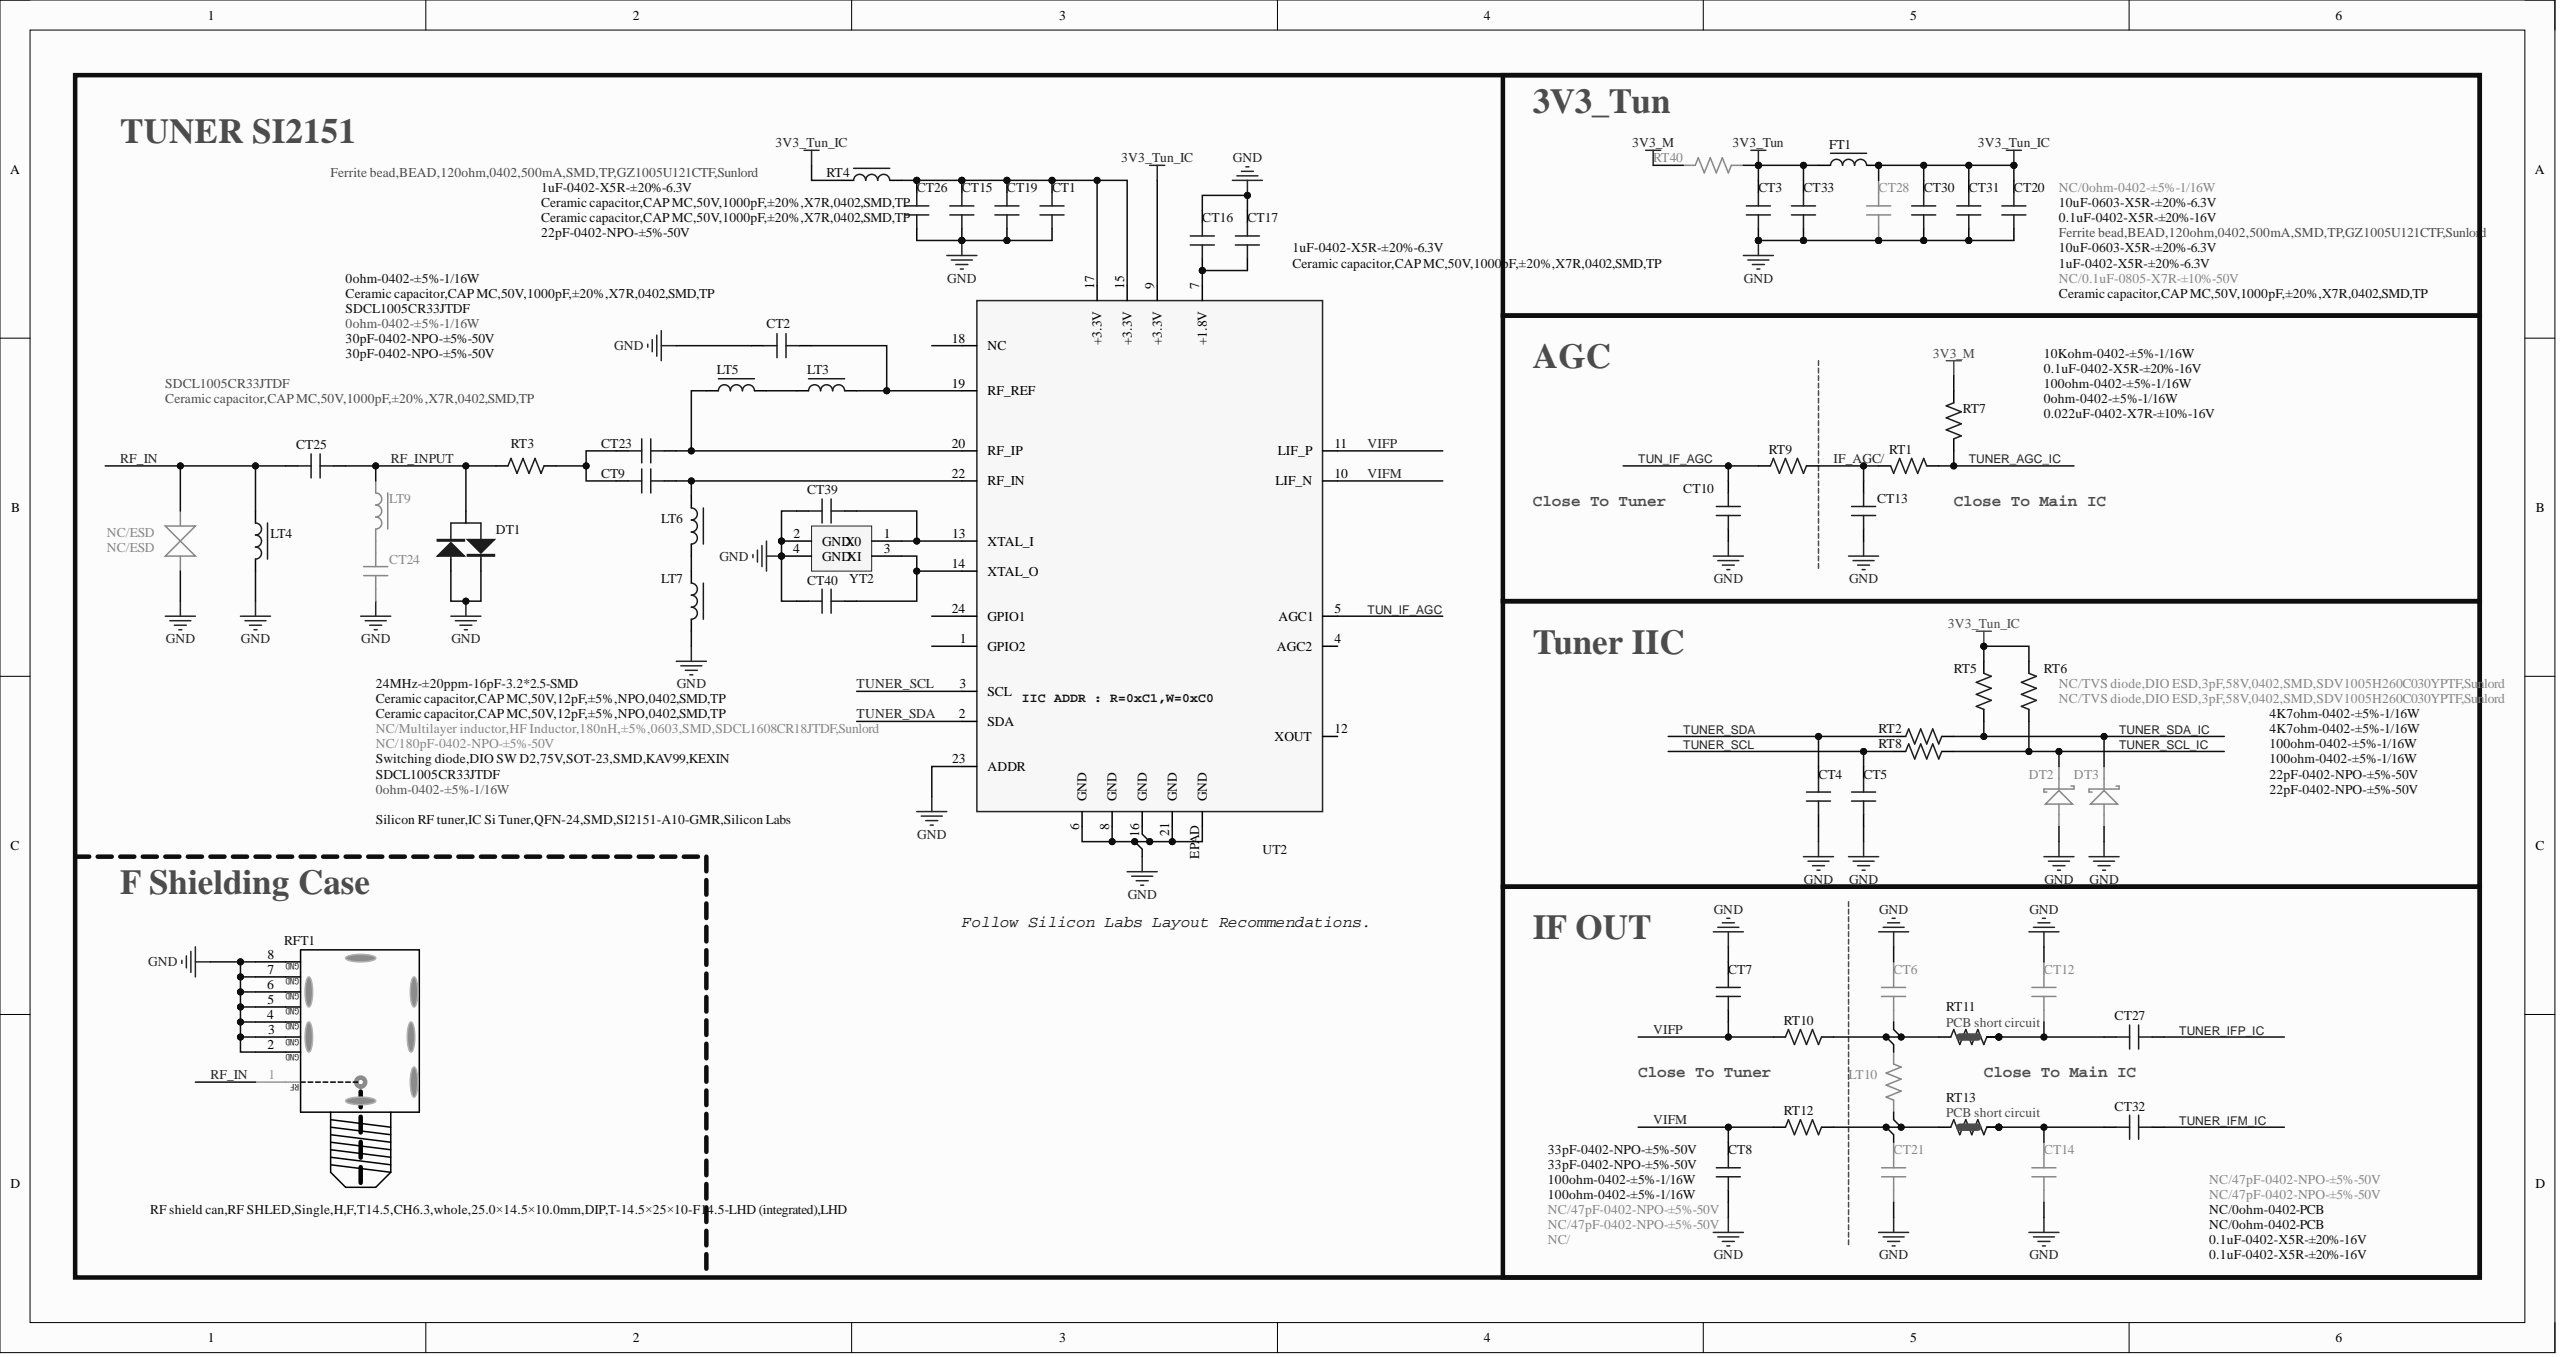Circuit board | Altium Designer | 1029 parts | 642 nets | one sheet of the schematic
Parts on this sheet (reference | value | footprint):
CT1 | Ceramic capacitor,CAP MC,50V,1000pF,±20%,X7R,0402,SMD,TP | C0402
CT2 | Ceramic capacitor,CAP MC,50V,1000pF,±20%,X7R,0402,SMD,TP | C0402
CT3 | 10uF-0603-X5R-±20%-6.3V | C0603
CT4 | 22pF-0402-NPO-±5%-50V | C0402
CT5 | 22pF-0402-NPO-±5%-50V | C0402
CT6 | NC/47pF-0402-NPO-±5%-50V | C0402
CT7 | 33pF-0402-NPO-±5%-50V | C0402
CT8 | 33pF-0402-NPO-±5%-50V | C0402
CT9 | 30pF-0402-NPO-±5%-50V | C0402
CT10 | 0.1uF-0402-X5R-±20%-16V | C0402
CT12 | NC/47pF-0402-NPO-±5%-50V | C0402
CT13 | 0.022uF-0402-X7R-±10%-16V | C0402
CT14 | NC/47pF-0402-NPO-±5%-50V | C0402
CT15 | 1uF-0402-X5R-±20%-6.3V | C0402
CT16 | 1uF-0402-X5R-±20%-6.3V | C0402
CT17 | Ceramic capacitor,CAP MC,50V,1000pF,±20%,X7R,0402,SMD,TP | C0402
CT19 | Ceramic capacitor,CAP MC,50V,1000pF,±20%,X7R,0402,SMD,TP | C0402
CT20 | Ceramic capacitor,CAP MC,50V,1000pF,±20%,X7R,0402,SMD,TP | C0402
CT21 | NC/47pF-0402-NPO-±5%-50V | C0402
CT23 | 30pF-0402-NPO-±5%-50V | C0402
CT24 | NC/180pF-0402-NPO-±5%-50V | C0402
CT25 | Ceramic capacitor,CAP MC,50V,1000pF,±20%,X7R,0402,SMD,TP | C0402
CT26 | 22pF-0402-NPO-±5%-50V | C0402
CT27 | 0.1uF-0402-X5R-±20%-16V | C0402
CT28 | NC/0.1uF-0805-X7R-±10%-50V | C0805
CT30 | 10uF-0603-X5R-±20%-6.3V | C0603
CT31 | 1uF-0402-X5R-±20%-6.3V | C0402
CT32 | 0.1uF-0402-X5R-±20%-16V | C0402
CT33 | 0.1uF-0402-X5R-±20%-16V | C0402
CT39 | Ceramic capacitor,CAP MC,50V,12pF,±5%,NPO,0402,SMD,TP | C0402
CT40 | Ceramic capacitor,CAP MC,50V,12pF,±5%,NPO,0402,SMD,TP | C0402
DT1 | Switching diode,DIO SW D2,75V,SOT-23,SMD,KAV99,KEXIN | SO-23
DT2 | NC/TVS diode,DIO ESD,3pF,58V,0402,SMD,SDV1005H260C030YPTF,Sunlord | DIODE-S0402
DT3 | NC/TVS diode,DIO ESD,3pF,58V,0402,SMD,SDV1005H260C030YPTF,Sunlord | DIODE-S0402
FT1 | Ferrite bead,BEAD,120ohm,0402,500mA,SMD,TP,GZ1005U121CTF,Sunlord | L0402
LT3 | 0ohm-0402-±5%-1/16W | L0402
LT4 | SDCL1005CR33JTDF | L0402
LT5 | SDCL1005CR33JTDF | L0402
LT6 | SDCL1005CR33JTDF | L0402
LT7 | 0ohm-0402-±5%-1/16W | L0402
LT9 | NC/Multilayer inductor,HF Inductor,180nH,±5%,0603,SMD,SDCL1608CR18JTDF,Sunlord | L0603
LT10 | NC/ | R0402
NC/ESD | NC/ESD | ESD
RFT1 | RF shield can,RF SHLED,Single,H,F,T14.5,CH6.3,whole,25.0×14.5×10.0mm,DIP,T-14.5×25×10-F14.5-LHD (integrated),LHD | T-14.5×25×10-F14.5-2
RT1 | 0ohm-0402-±5%-1/16W | R0402
RT2 | 100ohm-0402-±5%-1/16W | R0402
RT3 | 0ohm-0402-±5%-1/16W | R0402
RT4 | Ferrite bead,BEAD,120ohm,0402,500mA,SMD,TP,GZ1005U121CTF,Sunlord | L0402
RT5 | 4K7ohm-0402-±5%-1/16W | R0402
RT6 | 4K7ohm-0402-±5%-1/16W | R0402
RT7 | 10Kohm-0402-±5%-1/16W | R0402
RT8 | 100ohm-0402-±5%-1/16W | R0402
RT9 | 100ohm-0402-±5%-1/16W | R0402
RT10 | 100ohm-0402-±5%-1/16W | R0402
RT11 | NC/0ohm-0402-PCB | R0402SC
RT12 | 100ohm-0402-±5%-1/16W | R0402
RT13 | NC/0ohm-0402-PCB | R0402SC
RT40 | NC/0ohm-0402-±5%-1/16W | R0402
UT2 | Silicon RF tuner,IC Si Tuner,QFN-24,SMD,SI2151-A10-GMR,Silicon Labs | QFN24/0.4-1
YT2 | 24MHz-±20ppm-16pF-3.2*2.5-SMD | XTAL-S-3
Nets of these parts (net: part-pin ...):
VIFP: CT7-2 RT10-1 UT2-11
VIFM: CT8-2 RT12-1 UT2-10
TUNER_SDA_IC: DT3-K RT2-2 RT5-1
TUNER_SDA: CT4-1 RT2-1 UT2-2
TUNER_SCL_IC: DT2-K RT6-1 RT8-2
TUNER_SCL: CT5-1 RT8-1 UT2-3
TUNER_IFP_IC: CT27-1
TUNER_IFM_IC: CT32-2
TUNER_AGC_IC: RT1-2 RT7-1
TUN_IF_AGC: CT10-2 RT9-1 UT2-5
RF_INPUT: CT25-2 DT1-2 LT9-1 RT3-1
RF_IN: CT25-1 LT4-1 NC/ESD-2 RFT1-1
NetLT6_2: LT6-2 LT7-1
NetLT3_1: LT3-1 LT5-2
NetCT40_2: CT40-2 UT2-14 YT2-3
NetCT39_2: CT39-2 UT2-13 YT2-1
NetCT24_1: CT24-1 LT9-2
NetCT23_1: CT23-1 LT5-1 UT2-20
NetCT21_1: CT21-1 LT10-2 RT12-2 RT13-1
NetCT16_2: CT16-2 CT17-2 UT2-7
NetCT14_1: CT14-1 CT32-1 RT13-2 RT13-3
NetCT12_2: CT12-2 CT27-2 RT11-2 RT11-3
NetCT9_2: CT9-2 CT23-2 RT3-2
NetCT9_1: CT9-1 LT6-1 UT2-22
NetCT6_2: CT6-2 LT10-1 RT10-2 RT11-1
NetCT2_2: CT2-2 LT3-2 UT2-19
NetCT1_2: CT1-2 CT15-1 CT19-2 CT26-2 RT4-2 UT2-15 UT2-17
IF_AGC/: CT13-2 RT1-1 RT9-2
GND: CT1-1 CT2-1 CT3-1 CT4-2 CT5-2 CT6-1 CT7-1 CT8-1 CT10-1 CT12-1 CT13-1 CT14-2 CT15-2 CT16-1 CT17-1 CT19-1 CT20-1 CT21-2 CT24-2 CT26-1 CT28-1 CT30-1 CT31-1 CT33-1 CT39-1 CT40-1 DT1-1 DT1-3 DT2-A DT3-A LT4-2 LT7-2 NC/ESD-1 RFT1-2 RFT1-3 RFT1-4 RFT1-5 RFT1-6 RFT1-7 RFT1-8 UT2-6 UT2-8 UT2-16 UT2-21 UT2-23 UT2-EPAD YT2-2 YT2-4
3V3_Tun_IC: CT20-2 CT28-2 CT30-2 CT31-2 FT1-2 RT4-1 RT5-2 RT6-2 UT2-9
3V3_Tun: CT3-2 CT33-2 FT1-1 RT40-2
3V3_M: RT7-2 RT40-1